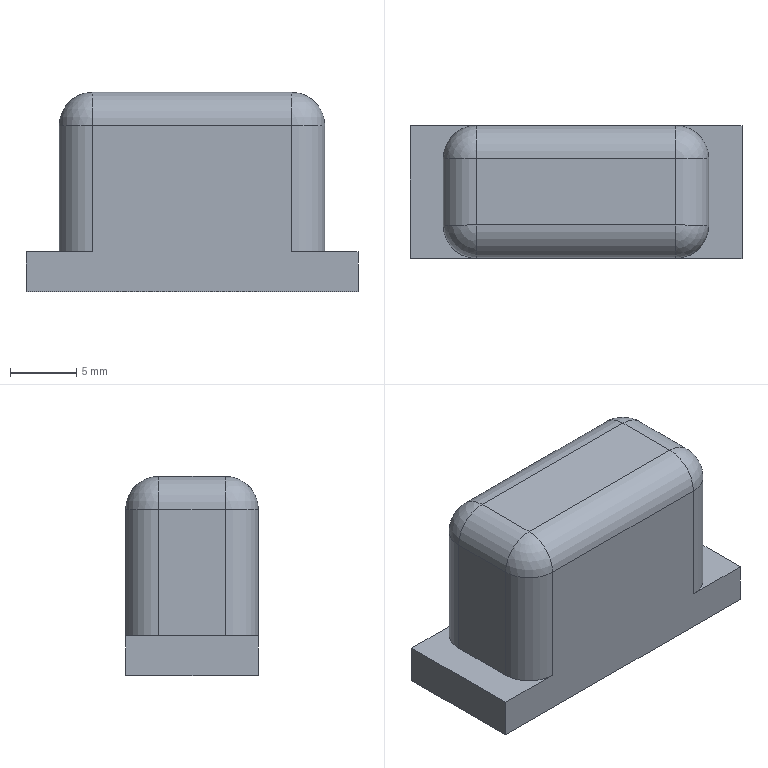NC program | NX | posted with a generic post | part box 25 x 10 x 15 mm
Lines 1 to 1365 of 3091:
N10 G17 G21 G94 G90
(FLOOR_WALL , TOOL : D50)
N12 T01 M6
N14 G54
N16 G17 G0 G90 X-42.5 Y0. S4000 M3
N18 G43 Z30. H1
N20 Z3.
N22 G94 G1 Z0. F1000.
N24 X-39.5
N26 X39.5
N28 X42.5
N30 Z3.
N32 G0 Z30.
N34 M5
(ZLEVEL_PROFILE , TOOL : D10)
N36 T10 M6
N38 G54
N40 G17 G0 G90 X-8.899 Y-8.585 S3500 M3
N42 G43 Z30. H10
N44 Z1.
N46 G94 G1 X-9.632 Y-8.378 Z0.96 F1000.
N48 X-10.462 Y-8.007 Z0.912
N50 X-11.23 Y-7.518 Z0.865
N52 X-11.919 Y-6.924 Z0.817
N54 X-12.515 Y-6.235 Z0.769
N56 X-13.004 Y-5.468 Z0.722
N58 X-13.376 Y-4.638 Z0.674
N60 X-13.624 Y-3.762 Z0.626
N62 X-13.743 Y-2.86 Z0.579
N64 Y-2.506 Z0.56
N66 Y2.506 Z0.297
N68 Y2.86 Z0.279
N70 X-13.624 Y3.762 Z0.231
N72 X-13.377 Y4.637 Z0.183
N74 X-13.005 Y5.467 Z0.136
N76 X-12.516 Y6.234 Z0.088
N78 X-11.921 Y6.922 Z0.04
N80 X-11.233 Y7.516 Z-0.007
N82 X-10.466 Y8.005 Z-0.055
N84 X-9.636 Y8.377 Z-0.103
N86 X-8.761 Y8.625 Z-0.15
N88 X-7.859 Y8.743 Z-0.198
N90 X-7.506 Z-0.216
N92 X7.506 F2500.
N94 G2 X13.743 Y2.5 R6.243
N96 G1 Y-2.5
N98 G2 X7.5 Y-8.743 R6.243
N100 G1 X-7.5
N102 G2 X-13.743 Y-2.506 R6.243
N104 G1 Y2.506
N106 G2 X-7.506 Y8.743 R6.243
N108 G1 X-7.284 Y8.75 Z-0.22
N110 X-7.063 Y8.757 Z-0.224
N112 X-6.842 Y8.764 Z-0.228
N114 X-6.62 Y8.771 Z-0.232
N116 X-6.399 Y8.778 Z-0.236
N118 X-6.178 Y8.785 Z-0.24
N120 X-5.956 Y8.791 Z-0.243
N122 X-5.735 Y8.798 Z-0.247
N124 X-5.514 Y8.805 Z-0.251
N126 X-5.292 Y8.811 Z-0.255
N128 X-5.071 Y8.818 Z-0.259
N130 X-4.85 Y8.825 Z-0.263
N132 X-4.628 Y8.831 Z-0.267
N134 X-4.407 Y8.838 Z-0.27
N136 X-4.185 Y8.844 Z-0.274
N138 X-3.964 Y8.85 Z-0.278
N140 X-3.743 Y8.857 Z-0.282
N142 X-3.521 Y8.863 Z-0.286
N144 X-3.3 Y8.869 Z-0.29
N146 X-3.079 Y8.875 Z-0.294
N148 X-2.857 Y8.882 Z-0.298
N150 X-2.636 Y8.888 Z-0.301
N152 X-2.415 Y8.894 Z-0.305
N154 X-2.193 Y8.9 Z-0.309
N156 X-1.972 Y8.906 Z-0.313
N158 X-1.751 Y8.912 Z-0.317
N160 X-1.529 Y8.918 Z-0.321
N162 X-1.308 Y8.924 Z-0.325
N164 X-1.087 Y8.93 Z-0.328
N166 X-0.865 Y8.936 Z-0.332
N168 X-0.644 Y8.941 Z-0.336
N170 X-0.423 Y8.947 Z-0.34
N172 X-0.201 Y8.953 Z-0.344
N174 X0.02 Y8.959 Z-0.348
N176 X0.241 Y8.964 Z-0.352
N178 X0.463 Y8.97 Z-0.355
N180 X0.684 Y8.976 Z-0.359
N182 X0.906 Y8.981 Z-0.363
N184 X1.127 Y8.987 Z-0.367
N186 X1.348 Y8.992 Z-0.371
N188 X1.57 Y8.998 Z-0.375
N190 X1.791 Y9.003 Z-0.379
N192 X2.012 Y9.009 Z-0.383
N194 X2.234 Y9.014 Z-0.386
N196 X2.455 Y9.019 Z-0.39
N198 X2.676 Y9.025 Z-0.394
N200 X2.898 Y9.03 Z-0.398
N202 X3.119 Y9.035 Z-0.402
N204 X3.34 Y9.041 Z-0.406
N206 X3.562 Y9.046 Z-0.41
N208 X3.783 Y9.051 Z-0.413
N210 X4.004 Y9.056 Z-0.417
N212 X4.226 Y9.062 Z-0.421
N214 X4.447 Y9.067 Z-0.425
N216 X4.668 Y9.072 Z-0.429
N218 X4.89 Y9.077 Z-0.433
N220 X7.506
N222 G2 X14.077 Y2.5 R6.577
N224 G1 Y-2.5
N226 G2 X7.5 Y-9.077 R6.577
N228 G1 X-7.5
N230 G2 X-14.077 Y-2.506 R6.577
N232 G1 Y2.506
N234 G2 X-7.506 Y9.077 R6.577
N236 G1 X-7.284 Y9.082 Z-0.437
N238 X-7.063 Y9.087 Z-0.44
N240 X-6.842 Y9.092 Z-0.444
N242 X-6.62 Y9.097 Z-0.448
N244 X-6.399 Y9.102 Z-0.452
N246 X-6.178 Y9.107 Z-0.456
N248 X-5.956 Y9.112 Z-0.46
N250 X-5.735 Y9.117 Z-0.464
N252 X-5.514 Y9.121 Z-0.468
N254 X-5.292 Y9.126 Z-0.471
N256 X-5.071 Y9.131 Z-0.475
N258 X-4.85 Y9.136 Z-0.479
N260 X-4.628 Y9.141 Z-0.483
N262 X-4.407 Y9.145 Z-0.487
N264 X-4.185 Y9.15 Z-0.491
N266 X-3.964 Y9.155 Z-0.495
N268 X-3.743 Y9.159 Z-0.498
N270 X-3.521 Y9.164 Z-0.502
N272 X-3.3 Y9.169 Z-0.506
N274 X-3.079 Y9.173 Z-0.51
N276 X-2.857 Y9.178 Z-0.514
N278 X-2.636 Y9.182 Z-0.518
N280 X-2.415 Y9.187 Z-0.522
N282 X-2.193 Y9.192 Z-0.525
N284 X-1.972 Y9.196 Z-0.529
N286 X-1.751 Y9.2 Z-0.533
N288 X-1.529 Y9.205 Z-0.537
N290 X-1.308 Y9.209 Z-0.541
N292 X-1.087 Y9.214 Z-0.545
N294 X-0.865 Y9.218 Z-0.549
N296 X-0.644 Y9.223 Z-0.553
N298 X-0.423 Y9.227 Z-0.556
N300 X-0.201 Y9.231 Z-0.56
N302 X0.02 Y9.236 Z-0.564
N304 X0.241 Y9.24 Z-0.568
N306 X0.463 Y9.244 Z-0.572
N308 X0.684 Y9.248 Z-0.576
N310 X0.906 Y9.253 Z-0.58
N312 X1.127 Y9.257 Z-0.583
N314 X1.348 Y9.261 Z-0.587
N316 X1.57 Y9.265 Z-0.591
N318 X1.791 Y9.269 Z-0.595
N320 X2.012 Y9.274 Z-0.599
N322 X2.234 Y9.278 Z-0.603
N324 X2.455 Y9.282 Z-0.607
N326 X2.676 Y9.286 Z-0.61
N328 X2.898 Y9.29 Z-0.614
N330 X3.119 Y9.294 Z-0.618
N332 X3.34 Y9.298 Z-0.622
N334 X3.562 Y9.302 Z-0.626
N336 X3.783 Y9.306 Z-0.63
N338 X4.004 Y9.31 Z-0.634
N340 X4.226 Y9.314 Z-0.638
N342 X4.447 Y9.318 Z-0.641
N344 X4.668 Y9.322 Z-0.645
N346 X4.89 Y9.326 Z-0.649
N348 X7.506
N350 G2 X14.326 Y2.5 R6.826
N352 G1 Y-2.5
N354 G2 X7.5 Y-9.326 R6.826
N356 G1 X-7.5
N358 G2 X-14.326 Y-2.498 R6.826
N360 G1 Y2.498
N362 G2 X-7.506 Y9.326 R6.826
N364 G1 X-7.284 Y9.33 Z-0.653
N366 X-7.063 Y9.334 Z-0.657
N368 X-6.842 Y9.338 Z-0.661
N370 X-6.62 Y9.341 Z-0.665
N372 X-6.399 Y9.345 Z-0.668
N374 X-6.178 Y9.349 Z-0.672
N376 X-5.956 Y9.353 Z-0.676
N378 X-5.735 Y9.357 Z-0.68
N380 X-5.514 Y9.361 Z-0.684
N382 X-5.292 Y9.364 Z-0.688
N384 X-5.071 Y9.368 Z-0.692
N386 X-4.85 Y9.372 Z-0.695
N388 X-4.628 Y9.376 Z-0.699
N390 X-4.407 Y9.379 Z-0.703
N392 X-4.185 Y9.383 Z-0.707
N394 X-3.964 Y9.387 Z-0.711
N396 X-3.743 Y9.39 Z-0.715
N398 X-3.521 Y9.394 Z-0.719
N400 X-3.3 Y9.397 Z-0.723
N402 X-3.079 Y9.401 Z-0.726
N404 X-2.857 Y9.405 Z-0.73
N406 X-2.636 Y9.408 Z-0.734
N408 X-2.415 Y9.412 Z-0.738
N410 X-2.193 Y9.415 Z-0.742
N412 X-1.972 Y9.419 Z-0.746
N414 X-1.751 Y9.422 Z-0.75
N416 X-1.529 Y9.426 Z-0.753
N418 X-1.308 Y9.429 Z-0.757
N420 X-1.087 Y9.433 Z-0.761
N422 X-0.865 Y9.436 Z-0.765
N424 X-0.644 Y9.44 Z-0.769
N426 X-0.423 Y9.443 Z-0.773
N428 X-0.201 Y9.447 Z-0.777
N430 X0.02 Y9.45 Z-0.78
N432 X0.241 Y9.454 Z-0.784
N434 X0.463 Y9.457 Z-0.788
N436 X0.684 Y9.46 Z-0.792
N438 X0.906 Y9.464 Z-0.796
N440 X1.127 Y9.467 Z-0.8
N442 X1.348 Y9.47 Z-0.804
N444 X1.57 Y9.474 Z-0.808
N446 X1.791 Y9.477 Z-0.811
N448 X2.012 Y9.48 Z-0.815
N450 X2.234 Y9.484 Z-0.819
N452 X2.455 Y9.487 Z-0.823
N454 X2.676 Y9.49 Z-0.827
N456 X2.898 Y9.493 Z-0.831
N458 X3.119 Y9.497 Z-0.835
N460 X3.34 Y9.5 Z-0.838
N462 X3.562 Y9.503 Z-0.842
N464 X3.783 Y9.506 Z-0.846
N466 X4.004 Y9.509 Z-0.85
N468 X4.226 Y9.513 Z-0.854
N470 X4.447 Y9.516 Z-0.858
N472 X4.668 Y9.519 Z-0.862
N474 X4.89 Y9.522 Z-0.865
N476 X7.506
N478 G2 X14.522 Y2.5 R7.022
N480 G1 Y-2.5
N482 G2 X7.5 Y-9.522 R7.022
N484 G1 X-7.5
N486 G2 X-14.522 Y-2.503 R7.022
N488 G1 Y2.503
N490 G2 X-7.506 Y9.522 R7.022
N492 G1 X-7.284 Y9.525 Z-0.869
N494 X-7.063 Y9.528 Z-0.873
N496 X-6.842 Y9.531 Z-0.877
N498 X-6.62 Y9.534 Z-0.881
N500 X-6.399 Y9.537 Z-0.885
N502 X-6.178 Y9.54 Z-0.889
N504 X-5.956 Y9.544 Z-0.893
N506 X-5.735 Y9.547 Z-0.896
N508 X-5.514 Y9.55 Z-0.9
N510 X-5.292 Y9.553 Z-0.904
N512 X-5.071 Y9.556 Z-0.908
N514 X-4.85 Y9.559 Z-0.912
N516 X-4.628 Y9.562 Z-0.916
N518 X-4.407 Y9.565 Z-0.92
N520 X-4.185 Y9.567 Z-0.923
N522 X-3.964 Y9.57 Z-0.927
N524 X-3.743 Y9.573 Z-0.931
N526 X-3.521 Y9.576 Z-0.935
N528 X-3.3 Y9.579 Z-0.939
N530 X-3.079 Y9.582 Z-0.943
N532 X-2.857 Y9.585 Z-0.947
N534 X-2.636 Y9.588 Z-0.95
N536 X-2.415 Y9.591 Z-0.954
N538 X-2.193 Y9.594 Z-0.958
N540 X-1.972 Y9.596 Z-0.962
N542 X-1.751 Y9.599 Z-0.966
N544 X-1.529 Y9.602 Z-0.97
N546 X-1.308 Y9.605 Z-0.974
N548 X-1.087 Y9.608 Z-0.978
N550 X-0.865 Y9.61 Z-0.981
N552 X-0.644 Y9.613 Z-0.985
N554 X-0.423 Y9.616 Z-0.989
N556 X-0.201 Y9.619 Z-0.993
N558 X0.02 Y9.621 Z-0.997
N560 X0.241 Y9.624 Z-1.001
N562 X0.463 Y9.627 Z-1.005
N564 X0.684 Y9.63 Z-1.008
N566 X0.906 Y9.632 Z-1.012
N568 X1.127 Y9.635 Z-1.016
N570 X1.348 Y9.638 Z-1.02
N572 X1.57 Y9.64 Z-1.024
N574 X1.791 Y9.643 Z-1.028
N576 X2.012 Y9.646 Z-1.032
N578 X2.234 Y9.648 Z-1.035
N580 X2.455 Y9.651 Z-1.039
N582 X2.676 Y9.654 Z-1.043
N584 X2.898 Y9.656 Z-1.047
N586 X3.119 Y9.659 Z-1.051
N588 X3.34 Y9.661 Z-1.055
N590 X3.562 Y9.664 Z-1.059
N592 X3.783 Y9.666 Z-1.063
N594 X4.004 Y9.669 Z-1.066
N596 X4.226 Y9.672 Z-1.07
N598 X4.447 Y9.674 Z-1.074
N600 X4.668 Y9.677 Z-1.078
N602 X4.89 Y9.679 Z-1.082
N604 X7.506
N606 G2 X14.679 Y2.5 R7.179
N608 G1 Y-2.5
N610 G2 X7.5 Y-9.679 R7.179
N612 G1 X-7.5
N614 G2 X-14.679 Y-2.506 R7.179
N616 G1 Y2.506
N618 G2 X-7.506 Y9.679 R7.179
N620 G1 X-7.284 Y9.682 Z-1.086
N622 X-7.063 Y9.684 Z-1.09
N624 X-6.842 Y9.687 Z-1.093
N626 X-6.62 Y9.689 Z-1.097
N628 X-6.399 Y9.692 Z-1.101
N630 X-6.178 Y9.694 Z-1.105
N632 X-5.956 Y9.697 Z-1.109
N634 X-5.735 Y9.699 Z-1.113
N636 X-5.514 Y9.701 Z-1.117
N638 X-5.292 Y9.704 Z-1.12
N640 X-5.071 Y9.706 Z-1.124
N642 X-4.85 Y9.709 Z-1.128
N644 X-4.628 Y9.711 Z-1.132
N646 X-4.407 Y9.713 Z-1.136
N648 X-4.185 Y9.716 Z-1.14
N650 X-3.964 Y9.718 Z-1.144
N652 X-3.743 Y9.721 Z-1.148
N654 X-3.521 Y9.723 Z-1.151
N656 X-3.3 Y9.725 Z-1.155
N658 X-3.079 Y9.728 Z-1.159
N660 X-2.857 Y9.73 Z-1.163
N662 X-2.636 Y9.732 Z-1.167
N664 X-2.415 Y9.734 Z-1.171
N666 X-2.193 Y9.737 Z-1.175
N668 X-1.972 Y9.739 Z-1.178
N670 X-1.751 Y9.741 Z-1.182
N672 X-1.529 Y9.744 Z-1.186
N674 X-1.308 Y9.746 Z-1.19
N676 X-1.087 Y9.748 Z-1.194
N678 X-0.865 Y9.75 Z-1.198
N680 X-0.644 Y9.753 Z-1.202
N682 X-0.423 Y9.755 Z-1.205
N684 X-0.201 Y9.757 Z-1.209
N686 X0.02 Y9.759 Z-1.213
N688 X0.241 Y9.761 Z-1.217
N690 X0.463 Y9.764 Z-1.221
N692 X0.684 Y9.766 Z-1.225
N694 X0.906 Y9.768 Z-1.229
N696 X1.127 Y9.77 Z-1.233
N698 X1.348 Y9.772 Z-1.236
N700 X1.57 Y9.774 Z-1.24
N702 X1.791 Y9.777 Z-1.244
N704 X2.012 Y9.779 Z-1.248
N706 X2.234 Y9.781 Z-1.252
N708 X2.455 Y9.783 Z-1.256
N710 X2.676 Y9.785 Z-1.26
N712 X2.898 Y9.787 Z-1.263
N714 X3.119 Y9.789 Z-1.267
N716 X3.34 Y9.791 Z-1.271
N718 X3.562 Y9.793 Z-1.275
N720 X3.783 Y9.795 Z-1.279
N722 X4.004 Y9.797 Z-1.283
N724 X4.226 Y9.799 Z-1.287
N726 X4.447 Y9.802 Z-1.29
N728 X4.668 Y9.804 Z-1.294
N730 X4.89 Y9.806 Z-1.298
N732 X7.506
N734 G2 X14.806 Y2.5 R7.306
N736 G1 Y-2.5
N738 G2 X7.5 Y-9.806 R7.306
N740 G1 X-7.5
N742 G2 X-14.806 Y-2.502 R7.306
N744 G1 Y2.502
N746 G2 X-7.506 Y9.806 R7.306
N748 G1 X-7.284 Y9.808 Z-1.302
N750 X-7.063 Y9.81 Z-1.306
N752 X-6.842 Y9.812 Z-1.31
N754 X-6.62 Y9.814 Z-1.314
N756 X-6.399 Y9.816 Z-1.318
N758 X-6.178 Y9.818 Z-1.321
N760 X-5.956 Y9.819 Z-1.325
N762 X-5.735 Y9.821 Z-1.329
N764 X-5.514 Y9.823 Z-1.333
N766 X-5.292 Y9.825 Z-1.337
N768 X-5.071 Y9.827 Z-1.341
N770 X-4.85 Y9.829 Z-1.345
N772 X-4.628 Y9.831 Z-1.348
N774 X-4.407 Y9.833 Z-1.352
N776 X-4.185 Y9.835 Z-1.356
N778 X-3.964 Y9.837 Z-1.36
N780 X-3.743 Y9.839 Z-1.364
N782 X-3.521 Y9.841 Z-1.368
N784 X-3.3 Y9.842 Z-1.372
N786 X-3.079 Y9.844 Z-1.375
N788 X-2.857 Y9.846 Z-1.379
N790 X-2.636 Y9.848 Z-1.383
N792 X-2.415 Y9.85 Z-1.387
N794 X-2.193 Y9.852 Z-1.391
N796 X-1.972 Y9.853 Z-1.395
N798 X-1.751 Y9.855 Z-1.399
N800 X-1.529 Y9.857 Z-1.403
N802 X-1.308 Y9.859 Z-1.406
N804 X-1.087 Y9.861 Z-1.41
N806 X-0.865 Y9.862 Z-1.414
N808 X-0.644 Y9.864 Z-1.418
N810 X-0.423 Y9.866 Z-1.422
N812 X-0.201 Y9.868 Z-1.426
N814 X0.02 Y9.869 Z-1.43
N816 X0.241 Y9.871 Z-1.433
N818 X0.463 Y9.873 Z-1.437
N820 X0.684 Y9.875 Z-1.441
N822 X0.906 Y9.876 Z-1.445
N824 X1.127 Y9.878 Z-1.449
N826 X1.348 Y9.88 Z-1.453
N828 X1.57 Y9.881 Z-1.457
N830 X1.791 Y9.883 Z-1.46
N832 X2.012 Y9.885 Z-1.464
N834 X2.234 Y9.886 Z-1.468
N836 X2.455 Y9.888 Z-1.472
N838 X2.676 Y9.89 Z-1.476
N840 X2.898 Y9.891 Z-1.48
N842 X3.119 Y9.893 Z-1.484
N844 X3.34 Y9.895 Z-1.488
N846 X3.562 Y9.896 Z-1.491
N848 X3.783 Y9.898 Z-1.495
N850 X4.004 Y9.9 Z-1.499
N852 X4.226 Y9.901 Z-1.503
N854 X4.447 Y9.903 Z-1.507
N856 X4.668 Y9.904 Z-1.511
N858 X4.89 Y9.906 Z-1.515
N860 X7.506
N862 G2 X14.906 Y2.5 R7.406
N864 G1 Y-2.5
N866 G2 X7.5 Y-9.906 R7.406
N868 G1 X-7.5
N870 G2 X-14.906 Y-2.504 R7.406
N872 G1 Y2.504
N874 G2 X-7.506 Y9.906 R7.406
N876 G1 X-7.284 Y9.908 Z-1.518
N878 X-7.063 Y9.909 Z-1.522
N880 X-6.842 Y9.911 Z-1.526
N882 X-6.62 Y9.912 Z-1.53
N884 X-6.399 Y9.914 Z-1.534
N886 X-6.178 Y9.915 Z-1.538
N888 X-5.956 Y9.917 Z-1.542
N890 X-5.735 Y9.918 Z-1.545
N892 X-5.514 Y9.92 Z-1.549
N894 X-5.292 Y9.921 Z-1.553
N896 X-5.071 Y9.923 Z-1.557
N898 X-4.85 Y9.924 Z-1.561
N900 X-4.628 Y9.926 Z-1.565
N902 X-4.407 Y9.927 Z-1.569
N904 X-4.185 Y9.929 Z-1.573
N906 X-3.964 Y9.93 Z-1.576
N908 X-3.743 Y9.932 Z-1.58
N910 X-3.521 Y9.933 Z-1.584
N912 X-3.3 Y9.935 Z-1.588
N914 X-3.079 Y9.936 Z-1.592
N916 X-2.857 Y9.938 Z-1.596
N918 X-2.636 Y9.939 Z-1.6
N920 X-2.415 Y9.941 Z-1.603
N922 X-2.193 Y9.942 Z-1.607
N924 X-1.972 Y9.943 Z-1.611
N926 X-1.751 Y9.945 Z-1.615
N928 X-1.529 Y9.946 Z-1.619
N930 X-1.308 Y9.948 Z-1.623
N932 X-1.087 Y9.949 Z-1.627
N934 X-0.865 Y9.95 Z-1.63
N936 X-0.644 Y9.952 Z-1.634
N938 X-0.423 Y9.953 Z-1.638
N940 X-0.201 Y9.954 Z-1.642
N942 X0.02 Y9.956 Z-1.646
N944 X0.241 Y9.957 Z-1.65
N946 X0.463 Y9.958 Z-1.654
N948 X0.684 Y9.96 Z-1.658
N950 X0.906 Y9.961 Z-1.661
N952 X1.127 Y9.962 Z-1.665
N954 X1.348 Y9.964 Z-1.669
N956 X1.57 Y9.965 Z-1.673
N958 X1.791 Y9.966 Z-1.677
N960 X2.012 Y9.968 Z-1.681
N962 X2.234 Y9.969 Z-1.685
N964 X2.455 Y9.97 Z-1.688
N966 X2.676 Y9.971 Z-1.692
N968 X2.898 Y9.973 Z-1.696
N970 X3.119 Y9.974 Z-1.7
N972 X3.34 Y9.975 Z-1.704
N974 X3.562 Y9.976 Z-1.708
N976 X3.783 Y9.978 Z-1.712
N978 X4.004 Y9.979 Z-1.715
N980 X4.226 Y9.98 Z-1.719
N982 X4.447 Y9.981 Z-1.723
N984 X4.668 Y9.982 Z-1.727
N986 X4.89 Y9.984 Z-1.731
N988 X7.506
N990 G2 X14.984 Y2.5 R7.484
N992 G1 Y-2.5
N994 G2 X7.5 Y-9.984 R7.484
N996 G1 X-7.5
N998 G2 X-14.984 Y-2.505 R7.484
N1000 G1 Y2.505
N1002 G2 X-7.506 Y9.984 R7.484
N1004 G1 X-7.284 Y9.985 Z-1.735
N1006 X-7.063 Y9.986 Z-1.739
N1008 X-6.842 Y9.987 Z-1.743
N1010 X-6.62 Y9.988 Z-1.746
N1012 X-6.399 Y9.99 Z-1.75
N1014 X-6.178 Y9.991 Z-1.754
N1016 X-5.956 Y9.992 Z-1.758
N1018 X-5.735 Y9.993 Z-1.762
N1020 X-5.514 Y9.994 Z-1.766
N1022 X-5.292 Y9.995 Z-1.77
N1024 X-5.071 Y9.996 Z-1.773
N1026 X-4.85 Y9.998 Z-1.777
N1028 X-4.628 Y9.999 Z-1.781
N1030 X-4.407 Y10. Z-1.785
N1032 X-4.185 Y10.001 Z-1.789
N1034 X-3.964 Y10.002 Z-1.793
N1036 X-3.743 Y10.003 Z-1.797
N1038 X-3.521 Y10.004 Z-1.8
N1040 X-3.3 Y10.005 Z-1.804
N1042 X-3.079 Y10.006 Z-1.808
N1044 X-2.857 Y10.007 Z-1.812
N1046 X-2.636 Y10.008 Z-1.816
N1048 X-2.415 Y10.009 Z-1.82
N1050 X-2.193 Y10.01 Z-1.824
N1052 X-1.972 Y10.012 Z-1.828
N1054 X-1.751 Y10.013 Z-1.831
N1056 X-1.529 Y10.014 Z-1.835
N1058 X-1.308 Y10.015 Z-1.839
N1060 X-1.087 Y10.016 Z-1.843
N1062 X-0.865 Y10.017 Z-1.847
N1064 X-0.644 Y10.018 Z-1.851
N1066 X-0.423 Y10.019 Z-1.855
N1068 X-0.201 Y10.02 Z-1.858
N1070 X0.02 Y10.021 Z-1.862
N1072 X0.241 Y10.022 Z-1.866
N1074 X0.463 Y10.023 Z-1.87
N1076 X0.684 Z-1.874
N1078 X0.906 Y10.024 Z-1.878
N1080 X1.127 Y10.025 Z-1.882
N1082 X1.348 Y10.026 Z-1.885
N1084 X1.57 Y10.027 Z-1.889
N1086 X1.791 Y10.028 Z-1.893
N1088 X2.012 Y10.029 Z-1.897
N1090 X2.234 Y10.03 Z-1.901
N1092 X2.455 Y10.031 Z-1.905
N1094 X2.676 Y10.032 Z-1.909
N1096 X2.898 Y10.033 Z-1.913
N1098 X3.119 Y10.034 Z-1.916
N1100 X3.34 Y10.035 Z-1.92
N1102 X3.562 Z-1.924
N1104 X3.783 Y10.036 Z-1.928
N1106 X4.004 Y10.037 Z-1.932
N1108 X4.226 Y10.038 Z-1.936
N1110 X4.447 Y10.039 Z-1.94
N1112 X4.668 Y10.04 Z-1.943
N1114 X4.89 Y10.041 Z-1.947
N1116 X7.506
N1118 G2 X15.041 Y2.5 R7.541
N1120 G1 Y-2.5
N1122 G2 X7.5 Y-10.041 R7.541
N1124 G1 X-7.5
N1126 G2 X-15.041 Y-2.505 R7.541
N1128 G1 Y2.505
N1130 G2 X-7.506 Y10.041 R7.541
N1132 G1 X-7.284 Z-1.951
N1134 X-7.063 Y10.042 Z-1.955
N1136 X-6.842 Y10.043 Z-1.959
N1138 X-6.62 Y10.044 Z-1.963
N1140 X-6.399 Y10.045 Z-1.967
N1142 X-6.178 Y10.046 Z-1.97
N1144 X-5.956 Z-1.974
N1146 X-5.735 Y10.047 Z-1.978
N1148 X-5.514 Y10.048 Z-1.982
N1150 X-5.292 Y10.049 Z-1.986
N1152 X-5.071 Z-1.99
N1154 X-4.85 Y10.05 Z-1.994
N1156 X-4.628 Y10.051 Z-1.998
N1158 X-4.407 Y10.052 Z-2.001
N1160 X-4.185 Z-2.005
N1162 X-3.964 Y10.053 Z-2.009
N1164 X-3.743 Y10.054 Z-2.013
N1166 X-3.521 Y10.055 Z-2.017
N1168 X-3.3 Z-2.021
N1170 X-3.079 Y10.056 Z-2.025
N1172 X-2.857 Y10.057 Z-2.028
N1174 X-2.636 Y10.058 Z-2.032
N1176 X-2.415 Z-2.036
N1178 X-2.193 Y10.059 Z-2.04
N1180 X-1.972 Y10.06 Z-2.044
N1182 X-1.751 Z-2.048
N1184 X-1.529 Y10.061 Z-2.052
N1186 X-1.308 Y10.062 Z-2.055
N1188 X-1.087 Z-2.059
N1190 X-0.865 Y10.063 Z-2.063
N1192 X-0.644 Y10.064 Z-2.067
N1194 X-0.423 Z-2.071
N1196 X-0.201 Y10.065 Z-2.075
N1198 X0.02 Y10.066 Z-2.079
N1200 X0.241 Z-2.083
N1202 X0.463 Y10.067 Z-2.086
N1204 X0.684 Y10.068 Z-2.09
N1206 X0.906 Z-2.094
N1208 X1.127 Y10.069 Z-2.098
N1210 X1.348 Z-2.102
N1212 X1.57 Y10.07 Z-2.106
N1214 X1.791 Y10.071 Z-2.11
N1216 X2.012 Z-2.113
N1218 X2.234 Y10.072 Z-2.117
N1220 X2.455 Z-2.121
N1222 X2.676 Y10.073 Z-2.125
N1224 X2.898 Z-2.129
N1226 X3.119 Y10.074 Z-2.133
N1228 X3.34 Z-2.137
N1230 X3.562 Y10.075 Z-2.14
N1232 X3.783 Y10.076 Z-2.144
N1234 X4.004 Z-2.148
N1236 X4.226 Y10.077 Z-2.152
N1238 X4.447 Z-2.156
N1240 X4.668 Y10.078 Z-2.16
N1242 X4.89 Z-2.164
N1244 X7.506
N1246 G2 X15.078 Y2.5 R7.578
N1248 G1 Y-2.5
N1250 G2 X7.5 Y-10.078 R7.578
N1252 G1 X-7.5
N1254 G2 X-15.078 Y-2.506 R7.578
N1256 G1 Y2.506
N1258 G2 X-7.506 Y10.078 R7.578
N1260 G1 X-7.284 Y10.079 Z-2.168
N1262 X-7.063 Z-2.171
N1264 X-6.842 Y10.08 Z-2.175
N1266 X-6.62 Z-2.179
N1268 X-6.399 Y10.081 Z-2.183
N1270 X-6.178 Z-2.187
N1272 X-5.956 Y10.082 Z-2.191
N1274 X-5.735 Z-2.195
N1276 X-5.514 Z-2.198
N1278 X-5.292 Y10.083 Z-2.202
N1280 X-5.071 Z-2.206
N1282 X-4.85 Y10.084 Z-2.21
N1284 X-4.628 Z-2.214
N1286 X-4.407 Y10.085 Z-2.218
N1288 X-4.185 Z-2.222
N1290 X-3.964 Z-2.225
N1292 X-3.743 Y10.086 Z-2.229
N1294 X-3.521 Z-2.233
N1296 X-3.3 Y10.087 Z-2.237
N1298 X-3.079 Z-2.241
N1300 X-2.857 Z-2.245
N1302 X-2.636 Y10.088 Z-2.249
N1304 X-2.415 Z-2.253
N1306 X-2.193 Y10.089 Z-2.256
N1308 X-1.972 Z-2.26
N1310 X-1.751 Z-2.264
N1312 X-1.529 Y10.09 Z-2.268
N1314 X-1.308 Z-2.272
N1316 X-1.087 Z-2.276
N1318 X-0.865 Y10.091 Z-2.28
N1320 X-0.644 Z-2.283
N1322 X-0.423 Z-2.287
N1324 X-0.201 Y10.092 Z-2.291
N1326 X0.02 Z-2.295
N1328 X0.241 Z-2.299
N1330 X0.463 Y10.093 Z-2.303
N1332 X0.684 Z-2.307
N1334 X0.906 Z-2.31
N1336 X1.127 Z-2.314
N1338 X1.348 Y10.094 Z-2.318
N1340 X1.57 Z-2.322
N1342 X1.791 Z-2.326
N1344 X2.012 Z-2.33
N1346 X2.234 Y10.095 Z-2.334
N1348 X2.455 Z-2.338
N1350 X2.676 Z-2.341
N1352 X2.898 Z-2.345
N1354 X3.119 Y10.096 Z-2.349
N1356 X3.34 Z-2.353
N1358 X3.562 Z-2.357
N1360 X3.783 Z-2.361
N1362 X4.004 Z-2.365
N1364 X4.226 Y10.097 Z-2.368
N1366 X4.447 Z-2.372
N1368 X4.668 Z-2.376
N1370 X4.89 Z-2.38
N1372 X7.506
N1374 G2 X15.097 Y2.5 R7.597
N1376 G1 Y-2.5
N1378 G2 X7.5 Y-10.097 R7.597
N1380 G1 X-7.5
N1382 G2 X-15.097 Y-2.506 R7.597
N1384 G1 Y2.506
N1386 G2 X-7.506 Y10.097 R7.597
N1388 G1 X-7.284 Z-2.384
N1390 X-7.063 Y10.098 Z-2.388
N1392 X-6.842 Z-2.392
N1394 X-6.62 Z-2.395
N1396 X-6.399 Z-2.399
N1398 X-6.178 Z-2.403
N1400 X-5.956 Z-2.407
N1402 X-5.735 Z-2.411
N1404 X-5.514 Y10.099 Z-2.415
N1406 X-5.292 Z-2.419
N1408 X-5.071 Z-2.423
N1410 X-4.85 Z-2.426
N1412 X-4.628 Z-2.43
N1414 X-4.407 Z-2.434
N1416 X-4.185 Z-2.438
N1418 X-3.964 Z-2.442
N1420 X-3.743 Z-2.446
N1422 X-3.521 Y10.1 Z-2.45
N1424 X-3.3 Z-2.453
N1426 X-3.079 Z-2.457
N1428 X-2.857 Z-2.461
N1430 X-2.636 Z-2.465
N1432 X-2.415 Z-2.469
N1434 X-2.193 Z-2.473
N1436 X-1.972 Z-2.477
N1438 X-1.751 Z-2.48
N1440 X-1.529 Z-2.484
N1442 X-1.308 Z-2.488
N1444 X-1.087 Z-2.492
N1446 X-0.865 Z-2.496
N1448 X-0.644 Z-2.5
N1450 X4.89 Z-2.596
N1452 X7.5
N1454 G2 X15.1 Y2.5 R7.6
N1456 G1 Y-2.5
N1458 G2 X7.5 Y-10.1 R7.6
N1460 G1 X-7.5
N1462 G2 X-15.1 Y-2.5 R7.6
N1464 G1 Y2.5
N1466 G2 X-7.506 Y10.1 R7.6
N1468 G1 X-7.284 Z-2.6
N1470 X4.89 Z-2.813
N1472 X7.5
N1474 G2 X15.1 Y2.5 R7.6
N1476 G1 Y-2.5
N1478 G2 X7.5 Y-10.1 R7.6
N1480 G1 X-7.5
N1482 G2 X-15.1 Y-2.5 R7.6
N1484 G1 Y2.5
N1486 G2 X-7.506 Y10.1 R7.6
N1488 G1 X-7.284 Z-2.817
N1490 X4.89 Z-3.029
N1492 X7.5
N1494 G2 X15.1 Y2.5 R7.6
N1496 G1 Y-2.5
N1498 G2 X7.5 Y-10.1 R7.6
N1500 G1 X-7.5
N1502 G2 X-15.1 Y-2.5 R7.6
N1504 G1 Y2.5
N1506 G2 X-7.506 Y10.1 R7.6
N1508 G1 X-7.284 Z-3.033
N1510 X4.89 Z-3.245
N1512 X7.5
N1514 G2 X15.1 Y2.5 R7.6
N1516 G1 Y-2.5
N1518 G2 X7.5 Y-10.1 R7.6
N1520 G1 X-7.5
N1522 G2 X-15.1 Y-2.5 R7.6
N1524 G1 Y2.5
N1526 G2 X-7.506 Y10.1 R7.6
N1528 G1 X-7.284 Z-3.249
N1530 X4.89 Z-3.462
N1532 X7.5
N1534 G2 X15.1 Y2.5 R7.6
N1536 G1 Y-2.5
N1538 G2 X7.5 Y-10.1 R7.6
N1540 G1 X-7.5
N1542 G2 X-15.1 Y-2.5 R7.6
N1544 G1 Y2.5
N1546 G2 X-7.506 Y10.1 R7.6
N1548 G1 X-7.284 Z-3.466
N1550 X4.89 Z-3.678
N1552 X7.5
N1554 G2 X15.1 Y2.5 R7.6
N1556 G1 Y-2.5
N1558 G2 X7.5 Y-10.1 R7.6
N1560 G1 X-7.5
N1562 G2 X-15.1 Y-2.5 R7.6
N1564 G1 Y2.5
N1566 G2 X-7.506 Y10.1 R7.6
N1568 G1 X-7.284 Z-3.682
N1570 X4.89 Z-3.895
N1572 X7.5
N1574 G2 X15.1 Y2.5 R7.6
N1576 G1 Y-2.5
N1578 G2 X7.5 Y-10.1 R7.6
N1580 G1 X-7.5
N1582 G2 X-15.1 Y-2.5 R7.6
N1584 G1 Y2.5
N1586 G2 X-7.506 Y10.1 R7.6
N1588 G1 X-7.284 Z-3.898
N1590 X4.89 Z-4.111
N1592 X7.5
N1594 G2 X15.1 Y2.5 R7.6
N1596 G1 Y-2.5
N1598 G2 X7.5 Y-10.1 R7.6
N1600 G1 X-7.5
N1602 G2 X-15.1 Y-2.5 R7.6
N1604 G1 Y2.5
N1606 G2 X-7.506 Y10.1 R7.6
N1608 G1 X-7.284 Z-4.115
N1610 X4.89 Z-4.327
N1612 X7.5
N1614 G2 X15.1 Y2.5 R7.6
N1616 G1 Y-2.5
N1618 G2 X7.5 Y-10.1 R7.6
N1620 G1 X-7.5
N1622 G2 X-15.1 Y-2.5 R7.6
N1624 G1 Y2.5
N1626 G2 X-7.506 Y10.1 R7.6
N1628 G1 X-7.284 Z-4.331
N1630 X4.89 Z-4.544
N1632 X7.5
N1634 G2 X15.1 Y2.5 R7.6
N1636 G1 Y-2.5
N1638 G2 X7.5 Y-10.1 R7.6
N1640 G1 X-7.5
N1642 G2 X-15.1 Y-2.5 R7.6
N1644 G1 Y2.5
N1646 G2 X-7.506 Y10.1 R7.6
N1648 G1 X-7.284 Z-4.548
N1650 X4.89 Z-4.76
N1652 X7.5
N1654 G2 X15.1 Y2.5 R7.6
N1656 G1 Y-2.5
N1658 G2 X7.5 Y-10.1 R7.6
N1660 G1 X-7.5
N1662 G2 X-15.1 Y-2.5 R7.6
N1664 G1 Y2.5
N1666 G2 X-7.506 Y10.1 R7.6
N1668 G1 X-7.284 Z-4.764
N1670 X4.89 Z-4.976
N1672 X7.5
N1674 G2 X15.1 Y2.5 R7.6
N1676 G1 Y-2.5
N1678 G2 X7.5 Y-10.1 R7.6
N1680 G1 X-7.5
N1682 G2 X-15.1 Y-2.5 R7.6
N1684 G1 Y2.5
N1686 G2 X-7.506 Y10.1 R7.6
N1688 G1 X-7.284 Z-4.98
N1690 X4.89 Z-5.193
N1692 X7.5
N1694 G2 X15.1 Y2.5 R7.6
N1696 G1 Y-2.5
N1698 G2 X7.5 Y-10.1 R7.6
N1700 G1 X-7.5
N1702 G2 X-15.1 Y-2.5 R7.6
N1704 G1 Y2.5
N1706 G2 X-7.506 Y10.1 R7.6
N1708 G1 X-7.284 Z-5.197
N1710 X4.89 Z-5.409
N1712 X7.5
N1714 G2 X15.1 Y2.5 R7.6
N1716 G1 Y-2.5
N1718 G2 X7.5 Y-10.1 R7.6
N1720 G1 X-7.5
N1722 G2 X-15.1 Y-2.5 R7.6
N1724 G1 Y2.5
N1726 G2 X-7.506 Y10.1 R7.6
N1728 G1 X-7.284 Z-5.413
N1730 X4.89 Z-5.625
N1732 X7.5
N1734 G2 X15.1 Y2.5 R7.6
N1736 G1 Y-2.5
N1738 G2 X7.5 Y-10.1 R7.6
N1740 G1 X-7.5
N1742 G2 X-15.1 Y-2.5 R7.6
N1744 G1 Y2.5
N1746 G2 X-7.506 Y10.1 R7.6
N1748 G1 X-7.284 Z-5.629
N1750 X4.89 Z-5.842
N1752 X7.5
N1754 G2 X15.1 Y2.5 R7.6
N1756 G1 Y-2.5
N1758 G2 X7.5 Y-10.1 R7.6
N1760 G1 X-7.5
N1762 G2 X-15.1 Y-2.5 R7.6
N1764 G1 Y2.5
N1766 G2 X-7.506 Y10.1 R7.6
N1768 G1 X-7.284 Z-5.846
N1770 X4.89 Z-6.058
N1772 X7.5
N1774 G2 X15.1 Y2.5 R7.6
N1776 G1 Y-2.5
N1778 G2 X7.5 Y-10.1 R7.6
N1780 G1 X-7.5
N1782 G2 X-15.1 Y-2.5 R7.6
N1784 G1 Y2.5
N1786 G2 X-7.506 Y10.1 R7.6
N1788 G1 X-7.284 Z-6.062
N1790 X4.89 Z-6.275
N1792 X7.5
N1794 G2 X15.1 Y2.5 R7.6
N1796 G1 Y-2.5
N1798 G2 X7.5 Y-10.1 R7.6
N1800 G1 X-7.5
N1802 G2 X-15.1 Y-2.5 R7.6
N1804 G1 Y2.5
N1806 G2 X-7.506 Y10.1 R7.6
N1808 G1 X-7.284 Z-6.278
N1810 X4.89 Z-6.491
N1812 X7.5
N1814 G2 X15.1 Y2.5 R7.6
N1816 G1 Y-2.5
N1818 G2 X7.5 Y-10.1 R7.6
N1820 G1 X-7.5
N1822 G2 X-15.1 Y-2.5 R7.6
N1824 G1 Y2.5
N1826 G2 X-7.506 Y10.1 R7.6
N1828 G1 X-7.284 Z-6.495
N1830 X4.89 Z-6.707
N1832 X7.5
N1834 G2 X15.1 Y2.5 R7.6
N1836 G1 Y-2.5
N1838 G2 X7.5 Y-10.1 R7.6
N1840 G1 X-7.5
N1842 G2 X-15.1 Y-2.5 R7.6
N1844 G1 Y2.5
N1846 G2 X-7.506 Y10.1 R7.6
N1848 G1 X-7.284 Z-6.711
N1850 X4.89 Z-6.924
N1852 X7.5
N1854 G2 X15.1 Y2.5 R7.6
N1856 G1 Y-2.5
N1858 G2 X7.5 Y-10.1 R7.6
N1860 G1 X-7.5
N1862 G2 X-15.1 Y-2.5 R7.6
N1864 G1 Y2.5
N1866 G2 X-7.506 Y10.1 R7.6
N1868 G1 X-7.284 Z-6.928
N1870 X4.89 Z-7.14
N1872 X7.5
N1874 G2 X15.1 Y2.5 R7.6
N1876 G1 Y-2.5
N1878 G2 X7.5 Y-10.1 R7.6
N1880 G1 X-7.5
N1882 G2 X-15.1 Y-2.5 R7.6
N1884 G1 Y2.5
N1886 G2 X-7.506 Y10.1 R7.6
N1888 G1 X-7.284 Z-7.144
N1890 X4.89 Z-7.356
N1892 X7.5
N1894 G2 X15.1 Y2.5 R7.6
N1896 G1 Y-2.5
N1898 G2 X7.5 Y-10.1 R7.6
N1900 G1 X-7.5
N1902 G2 X-15.1 Y-2.5 R7.6
N1904 G1 Y2.5
N1906 G2 X-7.506 Y10.1 R7.6
N1908 G1 X-7.284 Z-7.36
N1910 X4.89 Z-7.573
N1912 X7.5
N1914 G2 X15.1 Y2.5 R7.6
N1916 G1 Y-2.5
N1918 G2 X7.5 Y-10.1 R7.6
N1920 G1 X-7.5
N1922 G2 X-15.1 Y-2.5 R7.6
N1924 G1 Y2.5
N1926 G2 X-7.506 Y10.1 R7.6
N1928 G1 X-7.284 Z-7.577
N1930 X4.89 Z-7.789
N1932 X7.5
N1934 G2 X15.1 Y2.5 R7.6
N1936 G1 Y-2.5
N1938 G2 X7.5 Y-10.1 R7.6
N1940 G1 X-7.5
N1942 G2 X-15.1 Y-2.5 R7.6
N1944 G1 Y2.5
N1946 G2 X-7.506 Y10.1 R7.6
N1948 G1 X-7.284 Z-7.793
N1950 X4.89 Z-8.005
N1952 X7.5
N1954 G2 X15.1 Y2.5 R7.6
N1956 G1 Y-2.5
N1958 G2 X7.5 Y-10.1 R7.6
N1960 G1 X-7.5
N1962 G2 X-15.1 Y-2.5 R7.6
N1964 G1 Y2.5
N1966 G2 X-7.506 Y10.1 R7.6
N1968 G1 X-7.284 Z-8.009
N1970 X4.89 Z-8.222
N1972 X7.5
N1974 G2 X15.1 Y2.5 R7.6
N1976 G1 Y-2.5
N1978 G2 X7.5 Y-10.1 R7.6
N1980 G1 X-7.5
N1982 G2 X-15.1 Y-2.5 R7.6
N1984 G1 Y2.5
N1986 G2 X-7.506 Y10.1 R7.6
N1988 G1 X-7.284 Z-8.226
N1990 X4.89 Z-8.438
N1992 X7.5
N1994 G2 X15.1 Y2.5 R7.6
N1996 G1 Y-2.5
N1998 G2 X7.5 Y-10.1 R7.6
N2000 G1 X-7.5
N2002 G2 X-15.1 Y-2.5 R7.6
N2004 G1 Y2.5
N2006 G2 X-7.506 Y10.1 R7.6
N2008 G1 X-7.284 Z-8.442
N2010 X4.89 Z-8.655
N2012 X7.5
N2014 G2 X15.1 Y2.5 R7.6
N2016 G1 Y-2.5
N2018 G2 X7.5 Y-10.1 R7.6
N2020 G1 X-7.5
N2022 G2 X-15.1 Y-2.5 R7.6
N2024 G1 Y2.5
N2026 G2 X-7.506 Y10.1 R7.6
N2028 G1 X-7.284 Z-8.658
N2030 X4.89 Z-8.871
N2032 X7.5
N2034 G2 X15.1 Y2.5 R7.6
N2036 G1 Y-2.5
N2038 G2 X7.5 Y-10.1 R7.6
N2040 G1 X-7.5
N2042 G2 X-15.1 Y-2.5 R7.6
N2044 G1 Y2.5
N2046 G2 X-7.506 Y10.1 R7.6
N2048 G1 X-7.284 Z-8.875
N2050 X4.89 Z-9.087
N2052 X7.5
N2054 G2 X15.1 Y2.5 R7.6
N2056 G1 Y-2.5
N2058 G2 X7.5 Y-10.1 R7.6
N2060 G1 X-7.5
N2062 G2 X-15.1 Y-2.5 R7.6
N2064 G1 Y2.5
N2066 G2 X-7.506 Y10.1 R7.6
N2068 G1 X-7.284 Z-9.091
N2070 X4.89 Z-9.304
N2072 X7.5
N2074 G2 X15.1 Y2.5 R7.6
N2076 G1 Y-2.5
N2078 G2 X7.5 Y-10.1 R7.6
N2080 G1 X-7.5
N2082 G2 X-15.1 Y-2.5 R7.6
N2084 G1 Y2.5
N2086 G2 X-7.506 Y10.1 R7.6
N2088 G1 X-7.284 Z-9.308
N2090 X4.89 Z-9.52
N2092 X7.5
N2094 G2 X15.1 Y2.5 R7.6
N2096 G1 Y-2.5
N2098 G2 X7.5 Y-10.1 R7.6
N2100 G1 X-7.5
N2102 G2 X-15.1 Y-2.5 R7.6
N2104 G1 Y2.5
N2106 G2 X-7.506 Y10.1 R7.6
N2108 G1 X-7.284 Z-9.524
N2110 X4.89 Z-9.736
N2112 X7.5
N2114 G2 X15.1 Y2.5 R7.6
N2116 G1 Y-2.5
N2118 G2 X7.5 Y-10.1 R7.6
N2120 G1 X-7.5
N2122 G2 X-15.1 Y-2.5 R7.6
N2124 G1 Y2.5
N2126 G2 X-7.506 Y10.1 R7.6
N2128 G1 X-7.284 Z-9.74
N2130 X4.89 Z-9.953
N2132 X7.5
N2134 G2 X15.1 Y2.5 R7.6
N2136 G1 Y-2.5
N2138 G2 X7.5 Y-10.1 R7.6
N2140 G1 X-7.5
N2142 G2 X-15.1 Y-2.5 R7.6
N2144 G1 Y2.5
N2146 G2 X-7.506 Y10.1 R7.6
N2148 G1 X-7.284 Z-9.957
N2150 X4.89 Z-10.169
N2152 X7.5
N2154 G2 X15.1 Y2.5 R7.6
N2156 G1 Y-2.5
N2158 G2 X7.5 Y-10.1 R7.6
N2160 G1 X-7.5
N2162 G2 X-15.1 Y-2.5 R7.6
N2164 G1 Y2.5
N2166 G2 X-7.506 Y10.1 R7.6
N2168 G1 X-7.284 Z-10.173
N2170 X4.89 Z-10.385
N2172 X7.5
N2174 G2 X15.1 Y2.5 R7.6
N2176 G1 Y-2.5
N2178 G2 X7.5 Y-10.1 R7.6
N2180 G1 X-7.5
N2182 G2 X-15.1 Y-2.5 R7.6
N2184 G1 Y2.5
N2186 G2 X-7.506 Y10.1 R7.6
N2188 G1 X-7.284 Z-10.389
N2190 X4.89 Z-10.602
N2192 X7.5
N2194 G2 X15.1 Y2.5 R7.6
N2196 G1 Y-2.5
N2198 G2 X7.5 Y-10.1 R7.6
N2200 G1 X-7.5
N2202 G2 X-15.1 Y-2.5 R7.6
N2204 G1 Y2.5
N2206 G2 X-7.506 Y10.1 R7.6
N2208 G1 X-7.284 Z-10.606
N2210 X4.89 Z-10.818
N2212 X7.5
N2214 G2 X15.1 Y2.5 R7.6
N2216 G1 Y-2.5
N2218 G2 X7.5 Y-10.1 R7.6
N2220 G1 X-7.5
N2222 G2 X-15.1 Y-2.5 R7.6
N2224 G1 Y2.5
N2226 G2 X-7.506 Y10.1 R7.6
N2228 G1 X-7.284 Z-10.822
N2230 X4.89 Z-11.035
N2232 X7.5
N2234 G2 X15.1 Y2.5 R7.6
N2236 G1 Y-2.5
N2238 G2 X7.5 Y-10.1 R7.6
N2240 G1 X-7.5
N2242 G2 X-15.1 Y-2.5 R7.6
N2244 G1 Y2.5
N2246 G2 X-7.506 Y10.1 R7.6
N2248 G1 X-7.284 Z-11.038
N2250 X4.89 Z-11.251
N2252 X7.5
N2254 G2 X15.1 Y2.5 R7.6
N2256 G1 Y-2.5
N2258 G2 X7.5 Y-10.1 R7.6
N2260 G1 X-7.5
N2262 G2 X-15.1 Y-2.5 R7.6
N2264 G1 Y2.5
N2266 G2 X-7.506 Y10.1 R7.6
N2268 G1 X-7.284 Z-11.255
N2270 X4.89 Z-11.467
N2272 X7.5
N2274 G2 X15.1 Y2.5 R7.6
N2276 G1 Y-2.5
N2278 G2 X7.5 Y-10.1 R7.6
N2280 G1 X-7.5
N2282 G2 X-15.1 Y-2.5 R7.6
N2284 G1 Y2.5
N2286 G2 X-7.506 Y10.1 R7.6
N2288 G1 X-7.284 Z-11.471
N2290 X4.89 Z-11.684
N2292 X7.5
N2294 G2 X15.1 Y2.5 R7.6
N2296 G1 Y-2.5
N2298 G2 X7.5 Y-10.1 R7.6
N2300 G1 X-7.5
N2302 G2 X-15.1 Y-2.5 R7.6
N2304 G1 Y2.5
N2306 G2 X-7.506 Y10.1 R7.6
N2308 G1 X-7.284 Z-11.688
N2310 X4.89 Z-11.9
N2312 X7.5
N2314 G2 X15.1 Y2.5 R7.6
N2316 G1 Y-2.5
N2318 G2 X7.5 Y-10.1 R7.6
N2320 G1 X-7.5
N2322 G2 X-15.1 Y-2.5 R7.6
N2324 G1 Y2.5
N2326 G2 X-7.506 Y10.1 R7.6
N2328 G1 X-7.286 Z-11.904
N2330 X4.334 Z-12.107
N2332 X12.5
N2334 G2 X17.6 Y5. R5.1
N2336 G1 Y-5.
N2338 G2 X12.5 Y-10.1 R5.1
N2340 G1 X-12.5
N2342 G2 X-17.6 Y-5. R5.1
N2344 G1 Y5.
N2346 G2 X-12.5 Y10.1 R5.1
N2348 G1 X-7.506
N2350 X4.334 Z-12.313
N2352 X12.5
N2354 G2 X17.6 Y5. R5.1
N2356 G1 Y-5.
N2358 G2 X12.5 Y-10.1 R5.1
N2360 G1 X-12.5
N2362 G2 X-17.6 Y-5. R5.1
N2364 G1 Y5.
N2366 G2 X-12.5 Y10.1 R5.1
N2368 G1 X-7.506
N2370 X4.334 Z-12.52
N2372 X12.5
N2374 G2 X17.6 Y5. R5.1
N2376 G1 Y-5.
N2378 G2 X12.5 Y-10.1 R5.1
N2380 G1 X-12.5
N2382 G2 X-17.6 Y-5. R5.1
N2384 G1 Y5.
N2386 G2 X-12.5 Y10.1 R5.1
N2388 G1 X-7.506
N2390 X4.334 Z-12.727
N2392 X12.5
N2394 G2 X17.6 Y5. R5.1
N2396 G1 Y-5.
N2398 G2 X12.5 Y-10.1 R5.1
N2400 G1 X-12.5
N2402 G2 X-17.6 Y-5. R5.1
N2404 G1 Y5.
N2406 G2 X-12.5 Y10.1 R5.1
N2408 G1 X-7.506
N2410 X4.334 Z-12.933
N2412 X12.5
N2414 G2 X17.6 Y5. R5.1
N2416 G1 Y-5.
N2418 G2 X12.5 Y-10.1 R5.1
N2420 G1 X-12.5
N2422 G2 X-17.6 Y-5. R5.1
N2424 G1 Y5.
N2426 G2 X-12.5 Y10.1 R5.1
N2428 G1 X-7.506
N2430 X4.334 Z-13.14
N2432 X12.5
N2434 G2 X17.6 Y5. R5.1
N2436 G1 Y-5.
N2438 G2 X12.5 Y-10.1 R5.1
N2440 G1 X-12.5
N2442 G2 X-17.6 Y-5. R5.1
N2444 G1 Y5.
N2446 G2 X-12.5 Y10.1 R5.1
N2448 G1 X-7.506
N2450 X4.334 Z-13.347
N2452 X12.5
N2454 G2 X17.6 Y5. R5.1
N2456 G1 Y-5.
N2458 G2 X12.5 Y-10.1 R5.1
N2460 G1 X-12.5
N2462 G2 X-17.6 Y-5. R5.1
N2464 G1 Y5.
N2466 G2 X-12.5 Y10.1 R5.1
N2468 G1 X-7.506
N2470 X4.334 Z-13.553
N2472 X12.5
N2474 G2 X17.6 Y5. R5.1
N2476 G1 Y-5.
N2478 G2 X12.5 Y-10.1 R5.1
N2480 G1 X-12.5
N2482 G2 X-17.6 Y-5. R5.1
N2484 G1 Y5.
N2486 G2 X-12.5 Y10.1 R5.1
N2488 G1 X-7.506
N2490 X4.334 Z-13.76
N2492 X12.5
N2494 G2 X17.6 Y5. R5.1
N2496 G1 Y-5.
N2498 G2 X12.5 Y-10.1 R5.1
N2500 G1 X-12.5
N2502 G2 X-17.6 Y-5. R5.1
N2504 G1 Y5.
N2506 G2 X-12.5 Y10.1 R5.1
N2508 G1 X-7.506
N2510 X4.334 Z-13.967
N2512 X12.5
N2514 G2 X17.6 Y5. R5.1
N2516 G1 Y-5.
N2518 G2 X12.5 Y-10.1 R5.1
N2520 G1 X-12.5
N2522 G2 X-17.6 Y-5. R5.1
N2524 G1 Y5.
N2526 G2 X-12.5 Y10.1 R5.1
N2528 G1 X-7.506
N2530 X4.334 Z-14.173
N2532 X12.5
N2534 G2 X17.6 Y5. R5.1
N2536 G1 Y-5.
N2538 G2 X12.5 Y-10.1 R5.1
N2540 G1 X-12.5
N2542 G2 X-17.6 Y-5. R5.1
N2544 G1 Y5.
N2546 G2 X-12.5 Y10.1 R5.1
N2548 G1 X-7.506
N2550 X4.334 Z-14.38
N2552 X12.5
N2554 G2 X17.6 Y5. R5.1
N2556 G1 Y-5.
N2558 G2 X12.5 Y-10.1 R5.1
N2560 G1 X-12.5
N2562 G2 X-17.6 Y-5. R5.1
N2564 G1 Y5.
N2566 G2 X-12.5 Y10.1 R5.1
N2568 G1 X-7.506
N2570 X4.334 Z-14.587
N2572 X12.5
N2574 G2 X17.6 Y5. R5.1
N2576 G1 Y-5.
N2578 G2 X12.5 Y-10.1 R5.1
N2580 G1 X-12.5
N2582 G2 X-17.6 Y-5. R5.1
N2584 G1 Y5.
N2586 G2 X-12.5 Y10.1 R5.1
N2588 G1 X-7.506
N2590 X4.334 Z-14.793
N2592 X12.5
N2594 G2 X17.6 Y5. R5.1
N2596 G1 Y-5.
N2598 G2 X12.5 Y-10.1 R5.1
N2600 G1 X-12.5
N2602 G2 X-17.6 Y-5. R5.1
N2604 G1 Y5.
N2606 G2 X-12.5 Y10.1 R5.1
N2608 G1 X-7.506
N2610 X4.334 Z-15.
N2612 X12.5
N2614 G2 X17.6 Y5. R5.1
N2616 G1 Y-5.
N2618 G2 X12.5 Y-10.1 R5.1
N2620 G1 X-12.5
N2622 G2 X-17.6 Y-5. R5.1
N2624 G1 Y5.
N2626 G2 X-12.5 Y10.1 R5.1
N2628 G1 X4.334
N2630 Z-14.
N2632 G0 Z30.
N2634 M5
(ZLEVEL_PROFILE_COPY , TOOL : D10JING)
N2636 T11 M6
N2638 G54
N2640 G17 G0 G90 X-14.122 Y11.809 S5000 M3
N2642 G43 Z30. H11
N2644 Z-14.
N2646 G94 G1 Z-15. F1000.
N2648 X-13.366 Y10.5
N2650 G3 X-12.5 Y10. R1.
N2652 G1 X12.5 F1200.
N2654 G2 X17.5 Y5. R5.
N2656 G1 Y-5.
N2658 G2 X12.5 Y-10. R5.
N2660 G1 X-12.5
N2662 G2 X-17.5 Y-5. R5.
N2664 G1 Y5.
N2666 G2 X-12.5 Y10. R5.
N2668 G3 X-11.634 Y10.5 R1.
N2670 G1 X-10.768 Y12.
N2672 Z-14.
N2674 G0 Z30.
(ZLEVEL_PROFILE_COPY_COPY , TOOL : D10JING)
N2676 X-9.149 Y11.856
N2678 Z-11.
N2680 G1 Z-12. F1000.
N2682 X-8.366 Y10.5
N2684 G3 X-7.5 Y10. R1.
N2686 G1 X7.5 F1200.
N2688 G2 X15. Y2.5 R7.5
N2690 G1 Y-2.5
N2692 G2 X7.5 Y-10. R7.5
N2694 G1 X-7.5
N2696 G2 X-15. Y-2.5 R7.5
N2698 G1 Y2.5
N2700 G2 X-7.5 Y10. R7.5
N2702 G3 X-6.634 Y10.5 R1.
N2704 G1 X-5.768 Y12.
N2706 Z-11.
N2708 G0 Z30.
N2710 M5